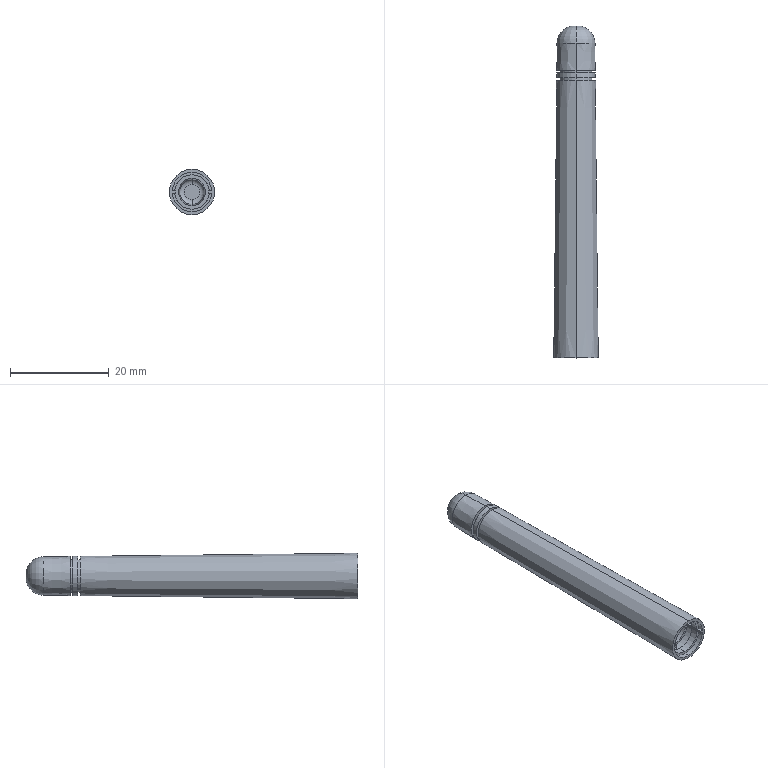Part | SolidWorks | features ICE 1, Revolution 1 | 1 solid | 62 faces | box 9.2 x 67.3 x 9.2 mm | volume 2059 mm3 | plane 27 | cylinder 23 | cone 8 | torus 4 | commonest cylinder face diameters 8 x11 7 x8 6.5 x4